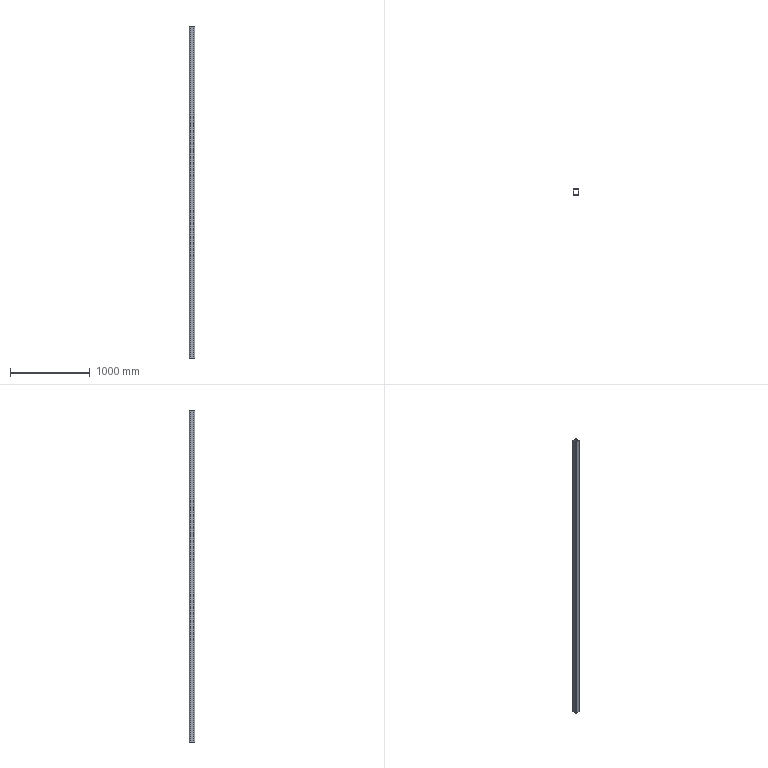Part | SolidWorks | features Extrusion 1 | 1 solid | 18 faces | box 70 x 70 x 4160 mm | volume 6004095 mm3 | plane 10 | cylinder 8 | commonest cylinder face diameters 12 x4 24 x4
STEP:
#1=CARTESIAN_POINT('',(0.,12.,4160.));
#2=VERTEX_POINT('',#1);
#3=CARTESIAN_POINT('',(12.,0.,4160.));
#4=VERTEX_POINT('',#3);
#5=CARTESIAN_POINT('',(12.,12.,4160.));
#6=DIRECTION('',(0.,0.,1.));
#7=DIRECTION('',(-1.,0.,0.));
#8=AXIS2_PLACEMENT_3D('',#5,#6,#7);
#9=CIRCLE('',#8,12.);
#10=EDGE_CURVE('',#2,#4,#9,.T.);
#11=ORIENTED_EDGE('',*,*,#10,.T.);
#12=CARTESIAN_POINT('',(58.,0.,4160.));
#13=VERTEX_POINT('',#12);
#14=CARTESIAN_POINT('',(12.,0.,4160.));
#15=DIRECTION('',(1.,0.,0.));
#16=VECTOR('',#15,1000.);
#17=LINE('',#14,#16);
#18=EDGE_CURVE('',#4,#13,#17,.T.);
#19=ORIENTED_EDGE('',*,*,#18,.T.);
#20=CARTESIAN_POINT('',(70.,12.,4160.));
#21=VERTEX_POINT('',#20);
#22=CARTESIAN_POINT('',(58.,12.,4160.));
#23=DIRECTION('',(0.,0.,1.));
#24=DIRECTION('',(1.,0.,0.));
#25=AXIS2_PLACEMENT_3D('',#22,#23,#24);
#26=CIRCLE('',#25,12.);
#27=EDGE_CURVE('',#13,#21,#26,.T.);
#28=ORIENTED_EDGE('',*,*,#27,.T.);
#29=CARTESIAN_POINT('',(70.,58.,4160.));
#30=VERTEX_POINT('',#29);
#31=CARTESIAN_POINT('',(70.,12.,4160.));
#32=DIRECTION('',(0.,1.,0.));
#33=VECTOR('',#32,1000.);
#34=LINE('',#31,#33);
#35=EDGE_CURVE('',#21,#30,#34,.T.);
#36=ORIENTED_EDGE('',*,*,#35,.T.);
#37=CARTESIAN_POINT('',(58.,70.,4160.));
#38=VERTEX_POINT('',#37);
#39=CARTESIAN_POINT('',(58.,58.,4160.));
#40=DIRECTION('',(0.,0.,1.));
#41=DIRECTION('',(-1.,0.,0.));
#42=AXIS2_PLACEMENT_3D('',#39,#40,#41);
#43=CIRCLE('',#42,12.);
#44=EDGE_CURVE('',#30,#38,#43,.T.);
#45=ORIENTED_EDGE('',*,*,#44,.T.);
#46=CARTESIAN_POINT('',(12.,70.,4160.));
#47=VERTEX_POINT('',#46);
#48=CARTESIAN_POINT('',(12.,70.,4160.));
#49=DIRECTION('',(-1.,0.,0.));
#50=VECTOR('',#49,1000.);
#51=LINE('',#48,#50);
#52=EDGE_CURVE('',#38,#47,#51,.T.);
#53=ORIENTED_EDGE('',*,*,#52,.T.);
#54=CARTESIAN_POINT('',(0.,58.,4160.));
#55=VERTEX_POINT('',#54);
#56=CARTESIAN_POINT('',(12.,58.,4160.));
#57=DIRECTION('',(0.,0.,1.));
#58=DIRECTION('',(-1.,0.,0.));
#59=AXIS2_PLACEMENT_3D('',#56,#57,#58);
#60=CIRCLE('',#59,12.);
#61=EDGE_CURVE('',#47,#55,#60,.T.);
#62=ORIENTED_EDGE('',*,*,#61,.T.);
#63=CARTESIAN_POINT('',(0.,12.,4160.));
#64=DIRECTION('',(0.,-1.,0.));
#65=VECTOR('',#64,1000.);
#66=LINE('',#63,#65);
#67=EDGE_CURVE('',#55,#2,#66,.T.);
#68=ORIENTED_EDGE('',*,*,#67,.T.);
#69=EDGE_LOOP('',(#11,#19,#28,#36,#45,#53,#62,#68));
#70=FACE_OUTER_BOUND('',#69,.T.);
#71=CARTESIAN_POINT('',(6.,12.,4160.));
#72=VERTEX_POINT('',#71);
#73=CARTESIAN_POINT('',(12.,6.,4160.));
#74=VERTEX_POINT('',#73);
#75=CARTESIAN_POINT('',(12.,12.,4160.));
#76=DIRECTION('',(0.,0.,1.));
#77=DIRECTION('',(-1.,0.,0.));
#78=AXIS2_PLACEMENT_3D('',#75,#76,#77);
#79=CIRCLE('',#78,6.);
#80=EDGE_CURVE('',#72,#74,#79,.T.);
#81=ORIENTED_EDGE('',*,*,#80,.F.);
#82=CARTESIAN_POINT('',(6.,58.,4160.));
#83=VERTEX_POINT('',#82);
#84=CARTESIAN_POINT('',(6.,12.,4160.));
#85=DIRECTION('',(0.,-1.,0.));
#86=VECTOR('',#85,1000.);
#87=LINE('',#84,#86);
#88=EDGE_CURVE('',#83,#72,#87,.T.);
#89=ORIENTED_EDGE('',*,*,#88,.F.);
#90=CARTESIAN_POINT('',(12.,64.,4160.));
#91=VERTEX_POINT('',#90);
#92=CARTESIAN_POINT('',(12.,58.,4160.));
#93=DIRECTION('',(0.,0.,1.));
#94=DIRECTION('',(-1.,0.,0.));
#95=AXIS2_PLACEMENT_3D('',#92,#93,#94);
#96=CIRCLE('',#95,6.);
#97=EDGE_CURVE('',#91,#83,#96,.T.);
#98=ORIENTED_EDGE('',*,*,#97,.F.);
#99=CARTESIAN_POINT('',(58.,64.,4160.));
#100=VERTEX_POINT('',#99);
#101=CARTESIAN_POINT('',(12.,64.,4160.));
#102=DIRECTION('',(-1.,0.,0.));
#103=VECTOR('',#102,1000.);
#104=LINE('',#101,#103);
#105=EDGE_CURVE('',#100,#91,#104,.T.);
#106=ORIENTED_EDGE('',*,*,#105,.F.);
#107=CARTESIAN_POINT('',(64.,58.,4160.));
#108=VERTEX_POINT('',#107);
#109=CARTESIAN_POINT('',(58.,58.,4160.));
#110=DIRECTION('',(0.,0.,1.));
#111=DIRECTION('',(-1.,0.,0.));
#112=AXIS2_PLACEMENT_3D('',#109,#110,#111);
#113=CIRCLE('',#112,6.);
#114=EDGE_CURVE('',#108,#100,#113,.T.);
#115=ORIENTED_EDGE('',*,*,#114,.F.);
#116=CARTESIAN_POINT('',(64.,12.,4160.));
#117=VERTEX_POINT('',#116);
#118=CARTESIAN_POINT('',(64.,12.,4160.));
#119=DIRECTION('',(0.,1.,0.));
#120=VECTOR('',#119,1000.);
#121=LINE('',#118,#120);
#122=EDGE_CURVE('',#117,#108,#121,.T.);
#123=ORIENTED_EDGE('',*,*,#122,.F.);
#124=CARTESIAN_POINT('',(58.,6.,4160.));
#125=VERTEX_POINT('',#124);
#126=CARTESIAN_POINT('',(58.,12.,4160.));
#127=DIRECTION('',(0.,0.,1.));
#128=DIRECTION('',(1.,0.,0.));
#129=AXIS2_PLACEMENT_3D('',#126,#127,#128);
#130=CIRCLE('',#129,6.);
#131=EDGE_CURVE('',#125,#117,#130,.T.);
#132=ORIENTED_EDGE('',*,*,#131,.F.);
#133=CARTESIAN_POINT('',(12.,6.,4160.));
#134=DIRECTION('',(1.,0.,0.));
#135=VECTOR('',#134,1000.);
#136=LINE('',#133,#135);
#137=EDGE_CURVE('',#74,#125,#136,.T.);
#138=ORIENTED_EDGE('',*,*,#137,.F.);
#139=EDGE_LOOP('',(#81,#89,#98,#106,#115,#123,#132,#138));
#140=FACE_BOUND('',#139,.T.);
#141=CARTESIAN_POINT('',(12.,12.,4160.));
#142=DIRECTION('',(0.,0.,-1.));
#143=DIRECTION('',(-1.,0.,0.));
#144=AXIS2_PLACEMENT_3D('',#141,#142,#143);
#145=PLANE('',#144);
#146=ADVANCED_FACE('',(#70,#140),#145,.F.);
#147=CARTESIAN_POINT('',(0.,12.,0.));
#148=VERTEX_POINT('',#147);
#149=CARTESIAN_POINT('',(12.,0.,0.));
#150=VERTEX_POINT('',#149);
#151=CARTESIAN_POINT('',(12.,12.,0.));
#152=DIRECTION('',(0.,0.,1.));
#153=DIRECTION('',(-1.,0.,0.));
#154=AXIS2_PLACEMENT_3D('',#151,#152,#153);
#155=CIRCLE('',#154,12.);
#156=EDGE_CURVE('',#148,#150,#155,.T.);
#157=ORIENTED_EDGE('',*,*,#156,.F.);
#158=CARTESIAN_POINT('',(0.,58.,0.));
#159=VERTEX_POINT('',#158);
#160=CARTESIAN_POINT('',(0.,12.,0.));
#161=DIRECTION('',(0.,-1.,0.));
#162=VECTOR('',#161,1000.);
#163=LINE('',#160,#162);
#164=EDGE_CURVE('',#159,#148,#163,.T.);
#165=ORIENTED_EDGE('',*,*,#164,.F.);
#166=CARTESIAN_POINT('',(12.,70.,0.));
#167=VERTEX_POINT('',#166);
#168=CARTESIAN_POINT('',(12.,58.,0.));
#169=DIRECTION('',(0.,0.,1.));
#170=DIRECTION('',(-1.,0.,0.));
#171=AXIS2_PLACEMENT_3D('',#168,#169,#170);
#172=CIRCLE('',#171,12.);
#173=EDGE_CURVE('',#167,#159,#172,.T.);
#174=ORIENTED_EDGE('',*,*,#173,.F.);
#175=CARTESIAN_POINT('',(58.,70.,0.));
#176=VERTEX_POINT('',#175);
#177=CARTESIAN_POINT('',(12.,70.,0.));
#178=DIRECTION('',(-1.,0.,0.));
#179=VECTOR('',#178,1000.);
#180=LINE('',#177,#179);
#181=EDGE_CURVE('',#176,#167,#180,.T.);
#182=ORIENTED_EDGE('',*,*,#181,.F.);
#183=CARTESIAN_POINT('',(70.,58.,0.));
#184=VERTEX_POINT('',#183);
#185=CARTESIAN_POINT('',(58.,58.,0.));
#186=DIRECTION('',(0.,0.,1.));
#187=DIRECTION('',(-1.,0.,0.));
#188=AXIS2_PLACEMENT_3D('',#185,#186,#187);
#189=CIRCLE('',#188,12.);
#190=EDGE_CURVE('',#184,#176,#189,.T.);
#191=ORIENTED_EDGE('',*,*,#190,.F.);
#192=CARTESIAN_POINT('',(70.,12.,0.));
#193=VERTEX_POINT('',#192);
#194=CARTESIAN_POINT('',(70.,12.,0.));
#195=DIRECTION('',(0.,1.,0.));
#196=VECTOR('',#195,1000.);
#197=LINE('',#194,#196);
#198=EDGE_CURVE('',#193,#184,#197,.T.);
#199=ORIENTED_EDGE('',*,*,#198,.F.);
#200=CARTESIAN_POINT('',(58.,0.,0.));
#201=VERTEX_POINT('',#200);
#202=CARTESIAN_POINT('',(58.,12.,0.));
#203=DIRECTION('',(0.,0.,1.));
#204=DIRECTION('',(1.,0.,0.));
#205=AXIS2_PLACEMENT_3D('',#202,#203,#204);
#206=CIRCLE('',#205,12.);
#207=EDGE_CURVE('',#201,#193,#206,.T.);
#208=ORIENTED_EDGE('',*,*,#207,.F.);
#209=CARTESIAN_POINT('',(12.,0.,0.));
#210=DIRECTION('',(1.,0.,0.));
#211=VECTOR('',#210,1000.);
#212=LINE('',#209,#211);
#213=EDGE_CURVE('',#150,#201,#212,.T.);
#214=ORIENTED_EDGE('',*,*,#213,.F.);
#215=EDGE_LOOP('',(#157,#165,#174,#182,#191,#199,#208,#214));
#216=FACE_OUTER_BOUND('',#215,.T.);
#217=CARTESIAN_POINT('',(6.,58.,0.));
#218=VERTEX_POINT('',#217);
#219=CARTESIAN_POINT('',(6.,12.,0.));
#220=VERTEX_POINT('',#219);
#221=CARTESIAN_POINT('',(6.,12.,0.));
#222=DIRECTION('',(0.,-1.,0.));
#223=VECTOR('',#222,1000.);
#224=LINE('',#221,#223);
#225=EDGE_CURVE('',#218,#220,#224,.T.);
#226=ORIENTED_EDGE('',*,*,#225,.T.);
#227=CARTESIAN_POINT('',(12.,6.,0.));
#228=VERTEX_POINT('',#227);
#229=CARTESIAN_POINT('',(12.,12.,0.));
#230=DIRECTION('',(0.,0.,1.));
#231=DIRECTION('',(-1.,0.,0.));
#232=AXIS2_PLACEMENT_3D('',#229,#230,#231);
#233=CIRCLE('',#232,6.);
#234=EDGE_CURVE('',#220,#228,#233,.T.);
#235=ORIENTED_EDGE('',*,*,#234,.T.);
#236=CARTESIAN_POINT('',(58.,6.,0.));
#237=VERTEX_POINT('',#236);
#238=CARTESIAN_POINT('',(12.,6.,0.));
#239=DIRECTION('',(1.,0.,0.));
#240=VECTOR('',#239,1000.);
#241=LINE('',#238,#240);
#242=EDGE_CURVE('',#228,#237,#241,.T.);
#243=ORIENTED_EDGE('',*,*,#242,.T.);
#244=CARTESIAN_POINT('',(64.,12.,0.));
#245=VERTEX_POINT('',#244);
#246=CARTESIAN_POINT('',(58.,12.,0.));
#247=DIRECTION('',(0.,0.,1.));
#248=DIRECTION('',(1.,0.,0.));
#249=AXIS2_PLACEMENT_3D('',#246,#247,#248);
#250=CIRCLE('',#249,6.);
#251=EDGE_CURVE('',#237,#245,#250,.T.);
#252=ORIENTED_EDGE('',*,*,#251,.T.);
#253=CARTESIAN_POINT('',(64.,58.,0.));
#254=VERTEX_POINT('',#253);
#255=CARTESIAN_POINT('',(64.,12.,0.));
#256=DIRECTION('',(0.,1.,0.));
#257=VECTOR('',#256,1000.);
#258=LINE('',#255,#257);
#259=EDGE_CURVE('',#245,#254,#258,.T.);
#260=ORIENTED_EDGE('',*,*,#259,.T.);
#261=CARTESIAN_POINT('',(58.,64.,0.));
#262=VERTEX_POINT('',#261);
#263=CARTESIAN_POINT('',(58.,58.,0.));
#264=DIRECTION('',(0.,0.,1.));
#265=DIRECTION('',(-1.,0.,0.));
#266=AXIS2_PLACEMENT_3D('',#263,#264,#265);
#267=CIRCLE('',#266,6.);
#268=EDGE_CURVE('',#254,#262,#267,.T.);
#269=ORIENTED_EDGE('',*,*,#268,.T.);
#270=CARTESIAN_POINT('',(12.,64.,0.));
#271=VERTEX_POINT('',#270);
#272=CARTESIAN_POINT('',(12.,64.,0.));
#273=DIRECTION('',(-1.,0.,0.));
#274=VECTOR('',#273,1000.);
#275=LINE('',#272,#274);
#276=EDGE_CURVE('',#262,#271,#275,.T.);
#277=ORIENTED_EDGE('',*,*,#276,.T.);
#278=CARTESIAN_POINT('',(12.,58.,0.));
#279=DIRECTION('',(0.,0.,1.));
#280=DIRECTION('',(-1.,0.,0.));
#281=AXIS2_PLACEMENT_3D('',#278,#279,#280);
#282=CIRCLE('',#281,6.);
#283=EDGE_CURVE('',#271,#218,#282,.T.);
#284=ORIENTED_EDGE('',*,*,#283,.T.);
#285=EDGE_LOOP('',(#226,#235,#243,#252,#260,#269,#277,#284));
#286=FACE_BOUND('',#285,.T.);
#287=CARTESIAN_POINT('',(12.,12.,0.));
#288=DIRECTION('',(0.,0.,-1.));
#289=DIRECTION('',(-1.,0.,0.));
#290=AXIS2_PLACEMENT_3D('',#287,#288,#289);
#291=PLANE('',#290);
#292=ADVANCED_FACE('',(#216,#286),#291,.T.);
#293=ORIENTED_EDGE('',*,*,#156,.T.);
#294=CARTESIAN_POINT('',(12.,0.,4160.));
#295=DIRECTION('',(0.,0.,-1.));
#296=VECTOR('',#295,1000.);
#297=LINE('',#294,#296);
#298=EDGE_CURVE('',#4,#150,#297,.T.);
#299=ORIENTED_EDGE('',*,*,#298,.F.);
#300=ORIENTED_EDGE('',*,*,#10,.F.);
#301=CARTESIAN_POINT('',(0.,12.,4160.));
#302=DIRECTION('',(0.,0.,-1.));
#303=VECTOR('',#302,1000.);
#304=LINE('',#301,#303);
#305=EDGE_CURVE('',#2,#148,#304,.T.);
#306=ORIENTED_EDGE('',*,*,#305,.T.);
#307=EDGE_LOOP('',(#293,#299,#300,#306));
#308=FACE_OUTER_BOUND('',#307,.T.);
#309=CARTESIAN_POINT('',(12.,12.,4160.));
#310=DIRECTION('',(0.,0.,-1.));
#311=DIRECTION('',(-1.,0.,0.));
#312=AXIS2_PLACEMENT_3D('',#309,#310,#311);
#313=CYLINDRICAL_SURFACE('',#312,12.);
#314=ADVANCED_FACE('',(#308),#313,.T.);
#315=ORIENTED_EDGE('',*,*,#213,.T.);
#316=CARTESIAN_POINT('',(58.,0.,4160.));
#317=DIRECTION('',(0.,0.,-1.));
#318=VECTOR('',#317,1000.);
#319=LINE('',#316,#318);
#320=EDGE_CURVE('',#13,#201,#319,.T.);
#321=ORIENTED_EDGE('',*,*,#320,.F.);
#322=ORIENTED_EDGE('',*,*,#18,.F.);
#323=ORIENTED_EDGE('',*,*,#298,.T.);
#324=EDGE_LOOP('',(#315,#321,#322,#323));
#325=FACE_OUTER_BOUND('',#324,.T.);
#326=CARTESIAN_POINT('',(12.,0.,4160.));
#327=DIRECTION('',(0.,1.,0.));
#328=DIRECTION('',(0.,0.,1.));
#329=AXIS2_PLACEMENT_3D('',#326,#327,#328);
#330=PLANE('',#329);
#331=ADVANCED_FACE('',(#325),#330,.F.);
#332=ORIENTED_EDGE('',*,*,#207,.T.);
#333=CARTESIAN_POINT('',(70.,12.,4160.));
#334=DIRECTION('',(0.,0.,-1.));
#335=VECTOR('',#334,1000.);
#336=LINE('',#333,#335);
#337=EDGE_CURVE('',#21,#193,#336,.T.);
#338=ORIENTED_EDGE('',*,*,#337,.F.);
#339=ORIENTED_EDGE('',*,*,#27,.F.);
#340=ORIENTED_EDGE('',*,*,#320,.T.);
#341=EDGE_LOOP('',(#332,#338,#339,#340));
#342=FACE_OUTER_BOUND('',#341,.T.);
#343=CARTESIAN_POINT('',(58.,12.,4160.));
#344=DIRECTION('',(0.,0.,-1.));
#345=DIRECTION('',(-1.,0.,0.));
#346=AXIS2_PLACEMENT_3D('',#343,#344,#345);
#347=CYLINDRICAL_SURFACE('',#346,12.);
#348=ADVANCED_FACE('',(#342),#347,.T.);
#349=ORIENTED_EDGE('',*,*,#198,.T.);
#350=CARTESIAN_POINT('',(70.,58.,4160.));
#351=DIRECTION('',(0.,0.,-1.));
#352=VECTOR('',#351,1000.);
#353=LINE('',#350,#352);
#354=EDGE_CURVE('',#30,#184,#353,.T.);
#355=ORIENTED_EDGE('',*,*,#354,.F.);
#356=ORIENTED_EDGE('',*,*,#35,.F.);
#357=ORIENTED_EDGE('',*,*,#337,.T.);
#358=EDGE_LOOP('',(#349,#355,#356,#357));
#359=FACE_OUTER_BOUND('',#358,.T.);
#360=CARTESIAN_POINT('',(70.,12.,4160.));
#361=DIRECTION('',(-1.,0.,0.));
#362=DIRECTION('',(0.,0.,1.));
#363=AXIS2_PLACEMENT_3D('',#360,#361,#362);
#364=PLANE('',#363);
#365=ADVANCED_FACE('',(#359),#364,.F.);
#366=ORIENTED_EDGE('',*,*,#190,.T.);
#367=CARTESIAN_POINT('',(58.,70.,4160.));
#368=DIRECTION('',(0.,0.,-1.));
#369=VECTOR('',#368,1000.);
#370=LINE('',#367,#369);
#371=EDGE_CURVE('',#38,#176,#370,.T.);
#372=ORIENTED_EDGE('',*,*,#371,.F.);
#373=ORIENTED_EDGE('',*,*,#44,.F.);
#374=ORIENTED_EDGE('',*,*,#354,.T.);
#375=EDGE_LOOP('',(#366,#372,#373,#374));
#376=FACE_OUTER_BOUND('',#375,.T.);
#377=CARTESIAN_POINT('',(58.,58.,4160.));
#378=DIRECTION('',(0.,0.,-1.));
#379=DIRECTION('',(-1.,0.,0.));
#380=AXIS2_PLACEMENT_3D('',#377,#378,#379);
#381=CYLINDRICAL_SURFACE('',#380,12.);
#382=ADVANCED_FACE('',(#376),#381,.T.);
#383=ORIENTED_EDGE('',*,*,#181,.T.);
#384=CARTESIAN_POINT('',(12.,70.,4160.));
#385=DIRECTION('',(0.,0.,-1.));
#386=VECTOR('',#385,1000.);
#387=LINE('',#384,#386);
#388=EDGE_CURVE('',#47,#167,#387,.T.);
#389=ORIENTED_EDGE('',*,*,#388,.F.);
#390=ORIENTED_EDGE('',*,*,#52,.F.);
#391=ORIENTED_EDGE('',*,*,#371,.T.);
#392=EDGE_LOOP('',(#383,#389,#390,#391));
#393=FACE_OUTER_BOUND('',#392,.T.);
#394=CARTESIAN_POINT('',(12.,70.,4160.));
#395=DIRECTION('',(0.,-1.,0.));
#396=DIRECTION('',(0.,0.,-1.));
#397=AXIS2_PLACEMENT_3D('',#394,#395,#396);
#398=PLANE('',#397);
#399=ADVANCED_FACE('',(#393),#398,.F.);
#400=ORIENTED_EDGE('',*,*,#173,.T.);
#401=CARTESIAN_POINT('',(0.,58.,4160.));
#402=DIRECTION('',(0.,0.,-1.));
#403=VECTOR('',#402,1000.);
#404=LINE('',#401,#403);
#405=EDGE_CURVE('',#55,#159,#404,.T.);
#406=ORIENTED_EDGE('',*,*,#405,.F.);
#407=ORIENTED_EDGE('',*,*,#61,.F.);
#408=ORIENTED_EDGE('',*,*,#388,.T.);
#409=EDGE_LOOP('',(#400,#406,#407,#408));
#410=FACE_OUTER_BOUND('',#409,.T.);
#411=CARTESIAN_POINT('',(12.,58.,4160.));
#412=DIRECTION('',(0.,0.,-1.));
#413=DIRECTION('',(-1.,0.,0.));
#414=AXIS2_PLACEMENT_3D('',#411,#412,#413);
#415=CYLINDRICAL_SURFACE('',#414,12.);
#416=ADVANCED_FACE('',(#410),#415,.T.);
#417=ORIENTED_EDGE('',*,*,#164,.T.);
#418=ORIENTED_EDGE('',*,*,#305,.F.);
#419=ORIENTED_EDGE('',*,*,#67,.F.);
#420=ORIENTED_EDGE('',*,*,#405,.T.);
#421=EDGE_LOOP('',(#417,#418,#419,#420));
#422=FACE_OUTER_BOUND('',#421,.T.);
#423=CARTESIAN_POINT('',(0.,12.,4160.));
#424=DIRECTION('',(1.,0.,0.));
#425=DIRECTION('',(0.,0.,-1.));
#426=AXIS2_PLACEMENT_3D('',#423,#424,#425);
#427=PLANE('',#426);
#428=ADVANCED_FACE('',(#422),#427,.F.);
#429=ORIENTED_EDGE('',*,*,#234,.F.);
#430=CARTESIAN_POINT('',(6.,12.,4160.));
#431=DIRECTION('',(0.,0.,-1.));
#432=VECTOR('',#431,1000.);
#433=LINE('',#430,#432);
#434=EDGE_CURVE('',#72,#220,#433,.T.);
#435=ORIENTED_EDGE('',*,*,#434,.F.);
#436=ORIENTED_EDGE('',*,*,#80,.T.);
#437=CARTESIAN_POINT('',(12.,6.,4160.));
#438=DIRECTION('',(0.,0.,-1.));
#439=VECTOR('',#438,1000.);
#440=LINE('',#437,#439);
#441=EDGE_CURVE('',#74,#228,#440,.T.);
#442=ORIENTED_EDGE('',*,*,#441,.T.);
#443=EDGE_LOOP('',(#429,#435,#436,#442));
#444=FACE_OUTER_BOUND('',#443,.T.);
#445=CARTESIAN_POINT('',(12.,12.,4160.));
#446=DIRECTION('',(0.,0.,-1.));
#447=DIRECTION('',(-1.,0.,0.));
#448=AXIS2_PLACEMENT_3D('',#445,#446,#447);
#449=CYLINDRICAL_SURFACE('',#448,6.);
#450=ADVANCED_FACE('',(#444),#449,.F.);
#451=ORIENTED_EDGE('',*,*,#242,.F.);
#452=ORIENTED_EDGE('',*,*,#441,.F.);
#453=ORIENTED_EDGE('',*,*,#137,.T.);
#454=CARTESIAN_POINT('',(58.,6.,4160.));
#455=DIRECTION('',(0.,0.,-1.));
#456=VECTOR('',#455,1000.);
#457=LINE('',#454,#456);
#458=EDGE_CURVE('',#125,#237,#457,.T.);
#459=ORIENTED_EDGE('',*,*,#458,.T.);
#460=EDGE_LOOP('',(#451,#452,#453,#459));
#461=FACE_OUTER_BOUND('',#460,.T.);
#462=CARTESIAN_POINT('',(12.,6.,4160.));
#463=DIRECTION('',(0.,1.,0.));
#464=DIRECTION('',(0.,0.,1.));
#465=AXIS2_PLACEMENT_3D('',#462,#463,#464);
#466=PLANE('',#465);
#467=ADVANCED_FACE('',(#461),#466,.T.);
#468=ORIENTED_EDGE('',*,*,#251,.F.);
#469=ORIENTED_EDGE('',*,*,#458,.F.);
#470=ORIENTED_EDGE('',*,*,#131,.T.);
#471=CARTESIAN_POINT('',(64.,12.,4160.));
#472=DIRECTION('',(0.,0.,-1.));
#473=VECTOR('',#472,1000.);
#474=LINE('',#471,#473);
#475=EDGE_CURVE('',#117,#245,#474,.T.);
#476=ORIENTED_EDGE('',*,*,#475,.T.);
#477=EDGE_LOOP('',(#468,#469,#470,#476));
#478=FACE_OUTER_BOUND('',#477,.T.);
#479=CARTESIAN_POINT('',(58.,12.,4160.));
#480=DIRECTION('',(0.,0.,-1.));
#481=DIRECTION('',(-1.,0.,0.));
#482=AXIS2_PLACEMENT_3D('',#479,#480,#481);
#483=CYLINDRICAL_SURFACE('',#482,6.);
#484=ADVANCED_FACE('',(#478),#483,.F.);
#485=ORIENTED_EDGE('',*,*,#259,.F.);
#486=ORIENTED_EDGE('',*,*,#475,.F.);
#487=ORIENTED_EDGE('',*,*,#122,.T.);
#488=CARTESIAN_POINT('',(64.,58.,4160.));
#489=DIRECTION('',(0.,0.,-1.));
#490=VECTOR('',#489,1000.);
#491=LINE('',#488,#490);
#492=EDGE_CURVE('',#108,#254,#491,.T.);
#493=ORIENTED_EDGE('',*,*,#492,.T.);
#494=EDGE_LOOP('',(#485,#486,#487,#493));
#495=FACE_OUTER_BOUND('',#494,.T.);
#496=CARTESIAN_POINT('',(64.,12.,4160.));
#497=DIRECTION('',(-1.,0.,0.));
#498=DIRECTION('',(0.,0.,1.));
#499=AXIS2_PLACEMENT_3D('',#496,#497,#498);
#500=PLANE('',#499);
#501=ADVANCED_FACE('',(#495),#500,.T.);
#502=ORIENTED_EDGE('',*,*,#268,.F.);
#503=ORIENTED_EDGE('',*,*,#492,.F.);
#504=ORIENTED_EDGE('',*,*,#114,.T.);
#505=CARTESIAN_POINT('',(58.,64.,4160.));
#506=DIRECTION('',(0.,0.,-1.));
#507=VECTOR('',#506,1000.);
#508=LINE('',#505,#507);
#509=EDGE_CURVE('',#100,#262,#508,.T.);
#510=ORIENTED_EDGE('',*,*,#509,.T.);
#511=EDGE_LOOP('',(#502,#503,#504,#510));
#512=FACE_OUTER_BOUND('',#511,.T.);
#513=CARTESIAN_POINT('',(58.,58.,4160.));
#514=DIRECTION('',(0.,0.,-1.));
#515=DIRECTION('',(-1.,0.,0.));
#516=AXIS2_PLACEMENT_3D('',#513,#514,#515);
#517=CYLINDRICAL_SURFACE('',#516,6.);
#518=ADVANCED_FACE('',(#512),#517,.F.);
#519=ORIENTED_EDGE('',*,*,#276,.F.);
#520=ORIENTED_EDGE('',*,*,#509,.F.);
#521=ORIENTED_EDGE('',*,*,#105,.T.);
#522=CARTESIAN_POINT('',(12.,64.,4160.));
#523=DIRECTION('',(0.,0.,-1.));
#524=VECTOR('',#523,1000.);
#525=LINE('',#522,#524);
#526=EDGE_CURVE('',#91,#271,#525,.T.);
#527=ORIENTED_EDGE('',*,*,#526,.T.);
#528=EDGE_LOOP('',(#519,#520,#521,#527));
#529=FACE_OUTER_BOUND('',#528,.T.);
#530=CARTESIAN_POINT('',(12.,64.,4160.));
#531=DIRECTION('',(0.,-1.,0.));
#532=DIRECTION('',(0.,0.,-1.));
#533=AXIS2_PLACEMENT_3D('',#530,#531,#532);
#534=PLANE('',#533);
#535=ADVANCED_FACE('',(#529),#534,.T.);
#536=ORIENTED_EDGE('',*,*,#283,.F.);
#537=ORIENTED_EDGE('',*,*,#526,.F.);
#538=ORIENTED_EDGE('',*,*,#97,.T.);
#539=CARTESIAN_POINT('',(6.,58.,4160.));
#540=DIRECTION('',(0.,0.,-1.));
#541=VECTOR('',#540,1000.);
#542=LINE('',#539,#541);
#543=EDGE_CURVE('',#83,#218,#542,.T.);
#544=ORIENTED_EDGE('',*,*,#543,.T.);
#545=EDGE_LOOP('',(#536,#537,#538,#544));
#546=FACE_OUTER_BOUND('',#545,.T.);
#547=CARTESIAN_POINT('',(12.,58.,4160.));
#548=DIRECTION('',(0.,0.,-1.));
#549=DIRECTION('',(-1.,0.,0.));
#550=AXIS2_PLACEMENT_3D('',#547,#548,#549);
#551=CYLINDRICAL_SURFACE('',#550,6.);
#552=ADVANCED_FACE('',(#546),#551,.F.);
#553=ORIENTED_EDGE('',*,*,#225,.F.);
#554=ORIENTED_EDGE('',*,*,#543,.F.);
#555=ORIENTED_EDGE('',*,*,#88,.T.);
#556=ORIENTED_EDGE('',*,*,#434,.T.);
#557=EDGE_LOOP('',(#553,#554,#555,#556));
#558=FACE_OUTER_BOUND('',#557,.T.);
#559=CARTESIAN_POINT('',(6.,12.,4160.));
#560=DIRECTION('',(1.,0.,0.));
#561=DIRECTION('',(0.,0.,-1.));
#562=AXIS2_PLACEMENT_3D('',#559,#560,#561);
#563=PLANE('',#562);
#564=ADVANCED_FACE('',(#558),#563,.T.);
#565=CLOSED_SHELL('',(#146,#292,#314,#331,#348,#365,#382,#399,#416,#428,#450,#467,#484,#501,#518,#535,#552,#564));
#566=MANIFOLD_SOLID_BREP('',#565);
#567=CARTESIAN_POINT('',(0.,0.,0.));
#568=DIRECTION('',(0.,0.,1.));
#569=DIRECTION('',(1.,0.,0.));
#570=AXIS2_PLACEMENT_3D('',#567,#568,#569);
#571=(LENGTH_UNIT()NAMED_UNIT(*)SI_UNIT(.MILLI.,.METRE.));
#572=UNCERTAINTY_MEASURE_WITH_UNIT(LENGTH_MEASURE(0.00001),#571,'','');
#573=(NAMED_UNIT(*)PLANE_ANGLE_UNIT()SI_UNIT($,.RADIAN.));
#574=(NAMED_UNIT(*)SI_UNIT($,.STERADIAN.)SOLID_ANGLE_UNIT());
#575=(GEOMETRIC_REPRESENTATION_CONTEXT(3)GLOBAL_UNCERTAINTY_ASSIGNED_CONTEXT((#572))GLOBAL_UNIT_ASSIGNED_CONTEXT((#571,#573,#574))REPRESENTATION_CONTEXT('',''));
#576=ADVANCED_BREP_SHAPE_REPRESENTATION('',(#566,#570),#575);